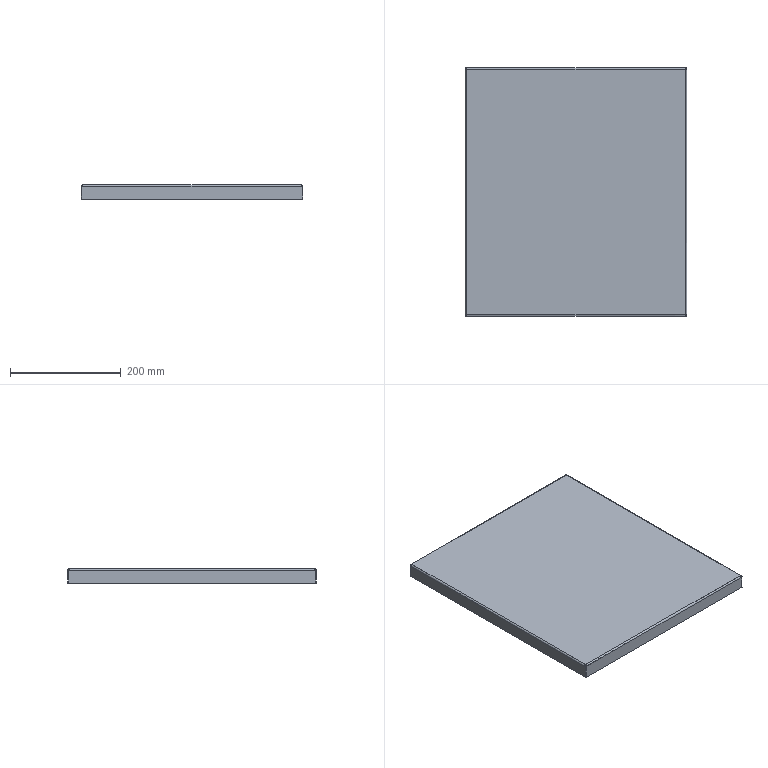Part | STEP file | Lower ctrl cover 1 | 1 solid | 70 faces | box 400 x 450 x 26 mm | volume 580163 mm3 | plane 26 | cylinder 24 | spline 20 | commonest cylinder face diameters 4 x8 1.473 x4 2 x4 5.473 x4 5 x2 9.5 x2